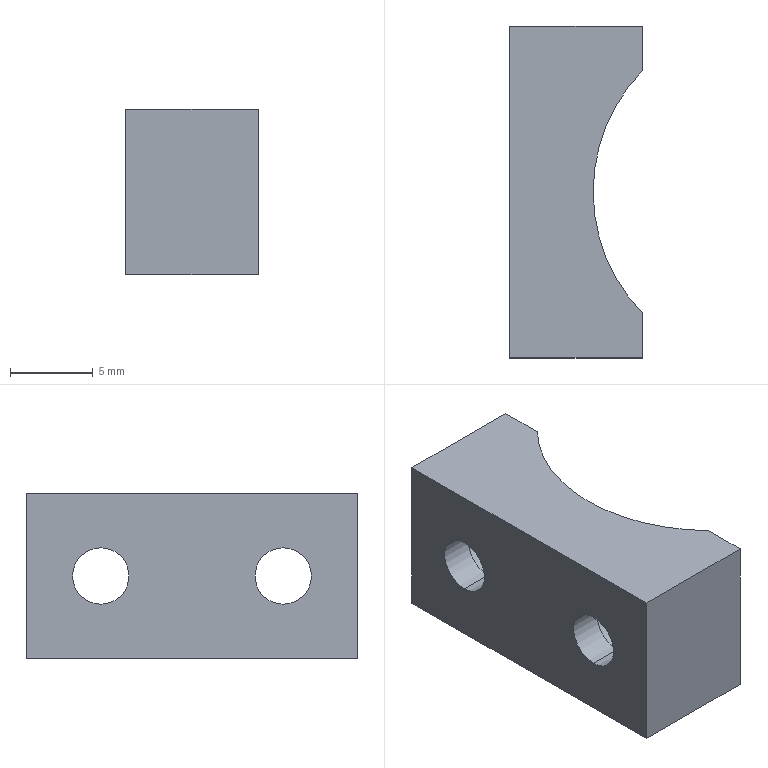Part | SolidWorks | features Extrusion 1, HoleWzd 1, RevCut 1 | 1 solid | 19 faces | box 8 x 20 x 10 mm | volume 974.548 mm3 | plane 9 | cylinder 8 | cone 2 | commonest cylinder face diameters 3.4 x4 6 x4
STEP:
#1=CARTESIAN_POINT('',(1.034,0.,10.));
#2=VERTEX_POINT('',#1);
#3=CARTESIAN_POINT('',(4.,7.299,10.));
#4=VERTEX_POINT('',#3);
#5=CARTESIAN_POINT('',(11.5,0.,10.));
#6=DIRECTION('',(0.,0.,-1.));
#7=DIRECTION('',(1.,0.,0.));
#8=AXIS2_PLACEMENT_3D('',#5,#6,#7);
#9=CIRCLE('',#8,10.466);
#10=EDGE_CURVE('',#2,#4,#9,.T.);
#11=ORIENTED_EDGE('',*,*,#10,.F.);
#12=CARTESIAN_POINT('',(0.5697,0.,0.));
#13=VERTEX_POINT('',#12);
#14=CARTESIAN_POINT('',(0.5,0.,-1.5));
#15=DIRECTION('',(-0.04641,0.,-0.9989));
#16=VECTOR('',#15,1000.);
#17=LINE('',#14,#16);
#18=EDGE_CURVE('',#2,#13,#17,.T.);
#19=ORIENTED_EDGE('',*,*,#18,.T.);
#20=CARTESIAN_POINT('',(4.,7.951,0.));
#21=VERTEX_POINT('',#20);
#22=CARTESIAN_POINT('',(11.5,0.,0.));
#23=DIRECTION('',(0.,0.,-1.));
#24=DIRECTION('',(1.,0.,0.));
#25=AXIS2_PLACEMENT_3D('',#22,#23,#24);
#26=CIRCLE('',#25,10.93);
#27=EDGE_CURVE('',#13,#21,#26,.T.);
#28=ORIENTED_EDGE('',*,*,#27,.T.);
#29=CARTESIAN_POINT('',(4.,7.757,3.024));
#30=VERTEX_POINT('',#29);
#31=CARTESIAN_POINT('',(4.,7.951,0.));
#32=CARTESIAN_POINT('',(4.,7.887,1.008));
#33=CARTESIAN_POINT('',(4.,7.822,2.016));
#34=CARTESIAN_POINT('',(4.,7.757,3.024));
#35=B_SPLINE_CURVE_WITH_KNOTS('',3,(#31,#32,#33,#34),.UNSPECIFIED.,.F.,.F.,(4,4),(0.0224,0.02543),.UNSPECIFIED.);
#36=EDGE_CURVE('',#21,#30,#35,.T.);
#37=ORIENTED_EDGE('',*,*,#36,.T.);
#38=CARTESIAN_POINT('',(2.162,5.5,2.));
#39=VERTEX_POINT('',#38);
#40=CARTESIAN_POINT('',(4.,7.757,3.024));
#41=CARTESIAN_POINT('',(3.843,7.616,2.863));
#42=CARTESIAN_POINT('',(3.684,7.463,2.722));
#43=CARTESIAN_POINT('',(3.365,7.131,2.473));
#44=CARTESIAN_POINT('',(3.204,6.952,2.366));
#45=CARTESIAN_POINT('',(2.887,6.568,2.188));
#46=CARTESIAN_POINT('',(2.733,6.367,2.12));
#47=CARTESIAN_POINT('',(2.439,5.948,2.026));
#48=CARTESIAN_POINT('',(2.297,5.729,2.));
#49=CARTESIAN_POINT('',(2.162,5.5,2.));
#50=B_SPLINE_CURVE_WITH_KNOTS('',3,(#40,#41,#42,#43,#44,#45,#46,#47,#48,#49),.UNSPECIFIED.,.F.,.F.,(4,2,2,2,4),(0.000000334,0.0007849,0.00157,0.002354,0.003139),.UNSPECIFIED.);
#51=EDGE_CURVE('',#30,#39,#50,.T.);
#52=ORIENTED_EDGE('',*,*,#51,.T.);
#53=CARTESIAN_POINT('',(2.487,5.5,8.));
#54=VERTEX_POINT('',#53);
#55=CARTESIAN_POINT('',(2.162,5.5,2.));
#56=CARTESIAN_POINT('',(2.057,5.322,2.));
#57=CARTESIAN_POINT('',(1.959,5.142,2.016));
#58=CARTESIAN_POINT('',(1.777,4.782,2.082));
#59=CARTESIAN_POINT('',(1.691,4.599,2.132));
#60=CARTESIAN_POINT('',(1.539,4.241,2.27));
#61=CARTESIAN_POINT('',(1.472,4.069,2.356));
#62=CARTESIAN_POINT('',(1.354,3.737,2.565));
#63=CARTESIAN_POINT('',(1.303,3.577,2.689));
#64=CARTESIAN_POINT('',(1.219,3.285,2.967));
#65=CARTESIAN_POINT('',(1.185,3.154,3.12));
#66=CARTESIAN_POINT('',(1.133,2.92,3.455));
#67=CARTESIAN_POINT('',(1.114,2.82,3.637));
#68=CARTESIAN_POINT('',(1.09,2.659,4.014));
#69=CARTESIAN_POINT('',(1.084,2.598,4.212));
#70=CARTESIAN_POINT('',(1.084,2.517,4.618));
#71=CARTESIAN_POINT('',(1.089,2.498,4.822));
#72=CARTESIAN_POINT('',(1.11,2.502,5.232));
#73=CARTESIAN_POINT('',(1.125,2.525,5.44));
#74=CARTESIAN_POINT('',(1.166,2.612,5.839));
#75=CARTESIAN_POINT('',(1.191,2.676,6.033));
#76=CARTESIAN_POINT('',(1.254,2.843,6.408));
#77=CARTESIAN_POINT('',(1.291,2.944,6.583));
#78=CARTESIAN_POINT('',(1.377,3.177,6.909));
#79=CARTESIAN_POINT('',(1.427,3.311,7.061));
#80=CARTESIAN_POINT('',(1.54,3.601,7.331));
#81=CARTESIAN_POINT('',(1.603,3.757,7.449));
#82=CARTESIAN_POINT('',(1.745,4.086,7.653));
#83=CARTESIAN_POINT('',(1.823,4.259,7.738));
#84=CARTESIAN_POINT('',(2.076,4.784,7.937));
#85=CARTESIAN_POINT('',(2.273,5.15,8.));
#86=CARTESIAN_POINT('',(2.487,5.5,8.));
#87=B_SPLINE_CURVE_WITH_KNOTS('',3,(#55,#56,#57,#58,#59,#60,#61,#62,#63,#64,#65,#66,#67,#68,#69,#70,#71,#72,#73,#74,#75,#76,#77,#78,#79,#80,#81,#82,#83,#84,#85,#86),.UNSPECIFIED.,.F.,.F.,(4,2,2,2,2,2,2,2,2,2,2,2,2,2,2,4),(0.003139,0.003751,0.004363,0.004975,0.005588,0.0062,0.006812,0.007424,0.008037,0.008649,0.009261,0.009873,0.01049,0.0111,0.01171,0.01293),.UNSPECIFIED.);
#88=EDGE_CURVE('',#39,#54,#87,.T.);
#89=ORIENTED_EDGE('',*,*,#88,.T.);
#90=CARTESIAN_POINT('',(4.,7.481,7.253));
#91=VERTEX_POINT('',#90);
#92=CARTESIAN_POINT('',(2.487,5.5,8.));
#93=CARTESIAN_POINT('',(2.601,5.687,8.));
#94=CARTESIAN_POINT('',(2.722,5.873,7.982));
#95=CARTESIAN_POINT('',(2.969,6.231,7.915));
#96=CARTESIAN_POINT('',(3.095,6.404,7.866));
#97=CARTESIAN_POINT('',(3.351,6.736,7.739));
#98=CARTESIAN_POINT('',(3.482,6.897,7.661));
#99=CARTESIAN_POINT('',(3.743,7.202,7.477));
#100=CARTESIAN_POINT('',(3.872,7.345,7.372));
#101=CARTESIAN_POINT('',(4.,7.481,7.253));
#102=B_SPLINE_CURVE_WITH_KNOTS('',3,(#92,#93,#94,#95,#96,#97,#98,#99,#100,#101),.UNSPECIFIED.,.F.,.F.,(4,2,2,2,4),(0.01293,0.01359,0.01424,0.0149,0.01555),.UNSPECIFIED.);
#103=EDGE_CURVE('',#54,#91,#102,.T.);
#104=ORIENTED_EDGE('',*,*,#103,.T.);
#105=CARTESIAN_POINT('',(4.,7.481,7.253));
#106=CARTESIAN_POINT('',(4.,7.421,8.168));
#107=CARTESIAN_POINT('',(4.,7.36,9.084));
#108=CARTESIAN_POINT('',(4.,7.299,10.));
#109=B_SPLINE_CURVE_WITH_KNOTS('',3,(#105,#106,#107,#108),.UNSPECIFIED.,.F.,.F.,(4,4),(0.02967,0.03242),.UNSPECIFIED.);
#110=EDGE_CURVE('',#91,#4,#109,.T.);
#111=ORIENTED_EDGE('',*,*,#110,.T.);
#112=EDGE_LOOP('',(#11,#19,#28,#37,#52,#89,#104,#111));
#113=FACE_OUTER_BOUND('',#112,.T.);
#114=CARTESIAN_POINT('',(11.5,0.,-1.5));
#115=DIRECTION('',(0.,0.,-1.));
#116=DIRECTION('',(-1.,0.,0.));
#117=AXIS2_PLACEMENT_3D('',#114,#115,#116);
#118=CONICAL_SURFACE('',#117,11.,0.04643);
#119=ADVANCED_FACE('',(#113),#118,.F.);
#120=CARTESIAN_POINT('',(-4.,5.5,6.7));
#121=VERTEX_POINT('',#120);
#122=CARTESIAN_POINT('',(-4.,5.5,3.3));
#123=VERTEX_POINT('',#122);
#124=CARTESIAN_POINT('',(-4.,5.5,5.));
#125=DIRECTION('',(1.,0.,0.));
#126=DIRECTION('',(0.,0.,-1.));
#127=AXIS2_PLACEMENT_3D('',#124,#125,#126);
#128=CIRCLE('',#127,1.7);
#129=EDGE_CURVE('',#121,#123,#128,.T.);
#130=ORIENTED_EDGE('',*,*,#129,.F.);
#131=CARTESIAN_POINT('',(-2.,5.5,6.7));
#132=VERTEX_POINT('',#131);
#133=CARTESIAN_POINT('',(4.,5.5,6.7));
#134=DIRECTION('',(1.,0.,0.));
#135=VECTOR('',#134,1000.);
#136=LINE('',#133,#135);
#137=EDGE_CURVE('',#121,#132,#136,.T.);
#138=ORIENTED_EDGE('',*,*,#137,.T.);
#139=CARTESIAN_POINT('',(-2.,5.5,3.3));
#140=VERTEX_POINT('',#139);
#141=CARTESIAN_POINT('',(-2.,5.5,5.));
#142=DIRECTION('',(1.,0.,0.));
#143=DIRECTION('',(0.,0.,-1.));
#144=AXIS2_PLACEMENT_3D('',#141,#142,#143);
#145=CIRCLE('',#144,1.7);
#146=EDGE_CURVE('',#132,#140,#145,.T.);
#147=ORIENTED_EDGE('',*,*,#146,.T.);
#148=CARTESIAN_POINT('',(4.,5.5,3.3));
#149=DIRECTION('',(1.,0.,0.));
#150=VECTOR('',#149,1000.);
#151=LINE('',#148,#150);
#152=EDGE_CURVE('',#123,#140,#151,.T.);
#153=ORIENTED_EDGE('',*,*,#152,.F.);
#154=EDGE_LOOP('',(#130,#138,#147,#153));
#155=FACE_OUTER_BOUND('',#154,.T.);
#156=CARTESIAN_POINT('',(4.,5.5,5.));
#157=DIRECTION('',(1.,0.,0.));
#158=DIRECTION('',(0.,0.,-1.));
#159=AXIS2_PLACEMENT_3D('',#156,#157,#158);
#160=CYLINDRICAL_SURFACE('',#159,1.7);
#161=ADVANCED_FACE('',(#155),#160,.F.);
#162=CARTESIAN_POINT('',(-4.,-5.5,6.7));
#163=VERTEX_POINT('',#162);
#164=CARTESIAN_POINT('',(-4.,-5.5,3.3));
#165=VERTEX_POINT('',#164);
#166=CARTESIAN_POINT('',(-4.,-5.5,5.));
#167=DIRECTION('',(1.,0.,0.));
#168=DIRECTION('',(0.,0.,-1.));
#169=AXIS2_PLACEMENT_3D('',#166,#167,#168);
#170=CIRCLE('',#169,1.7);
#171=EDGE_CURVE('',#163,#165,#170,.T.);
#172=ORIENTED_EDGE('',*,*,#171,.F.);
#173=CARTESIAN_POINT('',(-2.,-5.5,6.7));
#174=VERTEX_POINT('',#173);
#175=CARTESIAN_POINT('',(4.,-5.5,6.7));
#176=DIRECTION('',(1.,0.,0.));
#177=VECTOR('',#176,1000.);
#178=LINE('',#175,#177);
#179=EDGE_CURVE('',#163,#174,#178,.T.);
#180=ORIENTED_EDGE('',*,*,#179,.T.);
#181=CARTESIAN_POINT('',(-2.,-5.5,3.3));
#182=VERTEX_POINT('',#181);
#183=CARTESIAN_POINT('',(-2.,-5.5,5.));
#184=DIRECTION('',(1.,0.,0.));
#185=DIRECTION('',(0.,0.,-1.));
#186=AXIS2_PLACEMENT_3D('',#183,#184,#185);
#187=CIRCLE('',#186,1.7);
#188=EDGE_CURVE('',#174,#182,#187,.T.);
#189=ORIENTED_EDGE('',*,*,#188,.T.);
#190=CARTESIAN_POINT('',(4.,-5.5,3.3));
#191=DIRECTION('',(1.,0.,0.));
#192=VECTOR('',#191,1000.);
#193=LINE('',#190,#192);
#194=EDGE_CURVE('',#165,#182,#193,.T.);
#195=ORIENTED_EDGE('',*,*,#194,.F.);
#196=EDGE_LOOP('',(#172,#180,#189,#195));
#197=FACE_OUTER_BOUND('',#196,.T.);
#198=CARTESIAN_POINT('',(4.,-5.5,5.));
#199=DIRECTION('',(1.,0.,0.));
#200=DIRECTION('',(0.,0.,-1.));
#201=AXIS2_PLACEMENT_3D('',#198,#199,#200);
#202=CYLINDRICAL_SURFACE('',#201,1.7);
#203=ADVANCED_FACE('',(#197),#202,.F.);
#204=CARTESIAN_POINT('',(-2.,5.5,8.));
#205=VERTEX_POINT('',#204);
#206=CARTESIAN_POINT('',(-2.,5.5,2.));
#207=VERTEX_POINT('',#206);
#208=CARTESIAN_POINT('',(-2.,5.5,5.));
#209=DIRECTION('',(1.,0.,0.));
#210=DIRECTION('',(0.,0.,-1.));
#211=AXIS2_PLACEMENT_3D('',#208,#209,#210);
#212=CIRCLE('',#211,3.);
#213=EDGE_CURVE('',#205,#207,#212,.T.);
#214=ORIENTED_EDGE('',*,*,#213,.F.);
#215=CARTESIAN_POINT('',(4.,5.5,8.));
#216=DIRECTION('',(1.,0.,0.));
#217=VECTOR('',#216,1000.);
#218=LINE('',#215,#217);
#219=EDGE_CURVE('',#205,#54,#218,.T.);
#220=ORIENTED_EDGE('',*,*,#219,.T.);
#221=ORIENTED_EDGE('',*,*,#88,.F.);
#222=CARTESIAN_POINT('',(4.,5.5,2.));
#223=DIRECTION('',(1.,0.,0.));
#224=VECTOR('',#223,1000.);
#225=LINE('',#222,#224);
#226=EDGE_CURVE('',#207,#39,#225,.T.);
#227=ORIENTED_EDGE('',*,*,#226,.F.);
#228=EDGE_LOOP('',(#214,#220,#221,#227));
#229=FACE_OUTER_BOUND('',#228,.T.);
#230=CARTESIAN_POINT('',(4.,5.5,5.));
#231=DIRECTION('',(1.,0.,0.));
#232=DIRECTION('',(0.,0.,-1.));
#233=AXIS2_PLACEMENT_3D('',#230,#231,#232);
#234=CYLINDRICAL_SURFACE('',#233,3.);
#235=ADVANCED_FACE('',(#229),#234,.F.);
#236=CARTESIAN_POINT('',(-2.,-5.5,8.));
#237=VERTEX_POINT('',#236);
#238=CARTESIAN_POINT('',(-2.,-5.5,2.));
#239=VERTEX_POINT('',#238);
#240=CARTESIAN_POINT('',(-2.,-5.5,5.));
#241=DIRECTION('',(1.,0.,0.));
#242=DIRECTION('',(0.,0.,-1.));
#243=AXIS2_PLACEMENT_3D('',#240,#241,#242);
#244=CIRCLE('',#243,3.);
#245=EDGE_CURVE('',#237,#239,#244,.T.);
#246=ORIENTED_EDGE('',*,*,#245,.F.);
#247=CARTESIAN_POINT('',(2.487,-5.5,8.));
#248=VERTEX_POINT('',#247);
#249=CARTESIAN_POINT('',(4.,-5.5,8.));
#250=DIRECTION('',(1.,0.,0.));
#251=VECTOR('',#250,1000.);
#252=LINE('',#249,#251);
#253=EDGE_CURVE('',#237,#248,#252,.T.);
#254=ORIENTED_EDGE('',*,*,#253,.T.);
#255=CARTESIAN_POINT('',(4.,-7.481,7.253));
#256=VERTEX_POINT('',#255);
#257=CARTESIAN_POINT('',(4.,-7.481,7.253));
#258=CARTESIAN_POINT('',(3.743,-7.208,7.493));
#259=CARTESIAN_POINT('',(3.482,-6.906,7.674));
#260=CARTESIAN_POINT('',(3.094,-6.404,7.866));
#261=CARTESIAN_POINT('',(2.966,-6.228,7.916));
#262=CARTESIAN_POINT('',(2.72,-5.87,7.983));
#263=CARTESIAN_POINT('',(2.601,-5.687,8.));
#264=CARTESIAN_POINT('',(2.487,-5.5,8.));
#265=B_SPLINE_CURVE_WITH_KNOTS('',3,(#257,#258,#259,#260,#261,#262,#263,#264),.UNSPECIFIED.,.F.,.F.,(4,2,2,4),(0.000000342,0.001317,0.001975,0.002633),.UNSPECIFIED.);
#266=EDGE_CURVE('',#256,#248,#265,.T.);
#267=ORIENTED_EDGE('',*,*,#266,.F.);
#268=CARTESIAN_POINT('',(4.,-7.757,3.024));
#269=VERTEX_POINT('',#268);
#270=CARTESIAN_POINT('',(4.,-5.5,5.));
#271=DIRECTION('',(1.,0.,0.));
#272=DIRECTION('',(0.,0.,-1.));
#273=AXIS2_PLACEMENT_3D('',#270,#271,#272);
#274=CIRCLE('',#273,3.);
#275=EDGE_CURVE('',#256,#269,#274,.T.);
#276=ORIENTED_EDGE('',*,*,#275,.T.);
#277=CARTESIAN_POINT('',(2.162,-5.5,2.));
#278=VERTEX_POINT('',#277);
#279=CARTESIAN_POINT('',(2.162,-5.5,2.));
#280=CARTESIAN_POINT('',(2.295,-5.726,2.));
#281=CARTESIAN_POINT('',(2.437,-5.945,2.025));
#282=CARTESIAN_POINT('',(2.734,-6.368,2.12));
#283=CARTESIAN_POINT('',(2.889,-6.571,2.19));
#284=CARTESIAN_POINT('',(3.36,-7.139,2.453));
#285=CARTESIAN_POINT('',(3.688,-7.476,2.703));
#286=CARTESIAN_POINT('',(4.,-7.757,3.024));
#287=B_SPLINE_CURVE_WITH_KNOTS('',3,(#279,#280,#281,#282,#283,#284,#285,#286),.UNSPECIFIED.,.F.,.F.,(4,2,2,4),(0.01242,0.0132,0.01398,0.01554),.UNSPECIFIED.);
#288=EDGE_CURVE('',#278,#269,#287,.T.);
#289=ORIENTED_EDGE('',*,*,#288,.F.);
#290=CARTESIAN_POINT('',(4.,-5.5,2.));
#291=DIRECTION('',(1.,0.,0.));
#292=VECTOR('',#291,1000.);
#293=LINE('',#290,#292);
#294=EDGE_CURVE('',#239,#278,#293,.T.);
#295=ORIENTED_EDGE('',*,*,#294,.F.);
#296=EDGE_LOOP('',(#246,#254,#267,#276,#289,#295));
#297=FACE_OUTER_BOUND('',#296,.T.);
#298=CARTESIAN_POINT('',(4.,-5.5,5.));
#299=DIRECTION('',(1.,0.,0.));
#300=DIRECTION('',(0.,0.,-1.));
#301=AXIS2_PLACEMENT_3D('',#298,#299,#300);
#302=CYLINDRICAL_SURFACE('',#301,3.);
#303=ADVANCED_FACE('',(#297),#302,.F.);
#304=CARTESIAN_POINT('',(4.,-7.299,10.));
#305=VERTEX_POINT('',#304);
#306=CARTESIAN_POINT('',(4.,-7.299,10.));
#307=CARTESIAN_POINT('',(4.,-7.36,9.084));
#308=CARTESIAN_POINT('',(4.,-7.421,8.168));
#309=CARTESIAN_POINT('',(4.,-7.481,7.253));
#310=B_SPLINE_CURVE_WITH_KNOTS('',3,(#306,#307,#308,#309),.UNSPECIFIED.,.F.,.F.,(4,4),(0.02242,0.02517),.UNSPECIFIED.);
#311=EDGE_CURVE('',#305,#256,#310,.T.);
#312=ORIENTED_EDGE('',*,*,#311,.F.);
#313=CARTESIAN_POINT('',(4.,-10.,10.));
#314=VERTEX_POINT('',#313);
#315=CARTESIAN_POINT('',(4.,10.,10.));
#316=DIRECTION('',(0.,1.,0.));
#317=VECTOR('',#316,1000.);
#318=LINE('',#315,#317);
#319=EDGE_CURVE('',#314,#305,#318,.T.);
#320=ORIENTED_EDGE('',*,*,#319,.F.);
#321=CARTESIAN_POINT('',(4.,-10.,0.));
#322=VERTEX_POINT('',#321);
#323=CARTESIAN_POINT('',(4.,-10.,10.));
#324=DIRECTION('',(0.,0.,-1.));
#325=VECTOR('',#324,1000.);
#326=LINE('',#323,#325);
#327=EDGE_CURVE('',#314,#322,#326,.T.);
#328=ORIENTED_EDGE('',*,*,#327,.T.);
#329=CARTESIAN_POINT('',(4.,-7.951,0.));
#330=VERTEX_POINT('',#329);
#331=CARTESIAN_POINT('',(4.,10.,0.));
#332=DIRECTION('',(0.,1.,0.));
#333=VECTOR('',#332,1000.);
#334=LINE('',#331,#333);
#335=EDGE_CURVE('',#322,#330,#334,.T.);
#336=ORIENTED_EDGE('',*,*,#335,.T.);
#337=CARTESIAN_POINT('',(4.,-7.757,3.024));
#338=CARTESIAN_POINT('',(4.,-7.822,2.016));
#339=CARTESIAN_POINT('',(4.,-7.887,1.008));
#340=CARTESIAN_POINT('',(4.,-7.951,0.));
#341=B_SPLINE_CURVE_WITH_KNOTS('',3,(#337,#338,#339,#340),.UNSPECIFIED.,.F.,.F.,(4,4),(0.02941,0.03244),.UNSPECIFIED.);
#342=EDGE_CURVE('',#269,#330,#341,.T.);
#343=ORIENTED_EDGE('',*,*,#342,.F.);
#344=ORIENTED_EDGE('',*,*,#275,.F.);
#345=EDGE_LOOP('',(#312,#320,#328,#336,#343,#344));
#346=FACE_OUTER_BOUND('',#345,.T.);
#347=CARTESIAN_POINT('',(4.,10.,10.));
#348=DIRECTION('',(-1.,0.,0.));
#349=DIRECTION('',(0.,-1.,0.));
#350=AXIS2_PLACEMENT_3D('',#347,#348,#349);
#351=PLANE('',#350);
#352=ADVANCED_FACE('',(#346),#351,.F.);
#353=ORIENTED_EDGE('',*,*,#36,.F.);
#354=CARTESIAN_POINT('',(4.,10.,0.));
#355=VERTEX_POINT('',#354);
#356=CARTESIAN_POINT('',(4.,10.,0.));
#357=DIRECTION('',(0.,1.,0.));
#358=VECTOR('',#357,1000.);
#359=LINE('',#356,#358);
#360=EDGE_CURVE('',#21,#355,#359,.T.);
#361=ORIENTED_EDGE('',*,*,#360,.T.);
#362=CARTESIAN_POINT('',(4.,10.,10.));
#363=VERTEX_POINT('',#362);
#364=CARTESIAN_POINT('',(4.,10.,10.));
#365=DIRECTION('',(0.,0.,-1.));
#366=VECTOR('',#365,1000.);
#367=LINE('',#364,#366);
#368=EDGE_CURVE('',#363,#355,#367,.T.);
#369=ORIENTED_EDGE('',*,*,#368,.F.);
#370=CARTESIAN_POINT('',(4.,10.,10.));
#371=DIRECTION('',(0.,1.,0.));
#372=VECTOR('',#371,1000.);
#373=LINE('',#370,#372);
#374=EDGE_CURVE('',#4,#363,#373,.T.);
#375=ORIENTED_EDGE('',*,*,#374,.F.);
#376=ORIENTED_EDGE('',*,*,#110,.F.);
#377=CARTESIAN_POINT('',(4.,5.5,5.));
#378=DIRECTION('',(1.,0.,0.));
#379=DIRECTION('',(0.,0.,-1.));
#380=AXIS2_PLACEMENT_3D('',#377,#378,#379);
#381=CIRCLE('',#380,3.);
#382=EDGE_CURVE('',#30,#91,#381,.T.);
#383=ORIENTED_EDGE('',*,*,#382,.F.);
#384=EDGE_LOOP('',(#353,#361,#369,#375,#376,#383));
#385=FACE_OUTER_BOUND('',#384,.T.);
#386=CARTESIAN_POINT('',(4.,10.,10.));
#387=DIRECTION('',(-1.,0.,0.));
#388=DIRECTION('',(0.,-1.,0.));
#389=AXIS2_PLACEMENT_3D('',#386,#387,#388);
#390=PLANE('',#389);
#391=ADVANCED_FACE('',(#385),#390,.F.);
#392=ORIENTED_EDGE('',*,*,#253,.F.);
#393=CARTESIAN_POINT('',(-2.,-5.5,5.));
#394=DIRECTION('',(1.,0.,0.));
#395=DIRECTION('',(0.,0.,-1.));
#396=AXIS2_PLACEMENT_3D('',#393,#394,#395);
#397=CIRCLE('',#396,3.);
#398=EDGE_CURVE('',#239,#237,#397,.T.);
#399=ORIENTED_EDGE('',*,*,#398,.F.);
#400=ORIENTED_EDGE('',*,*,#294,.T.);
#401=CARTESIAN_POINT('',(2.487,-5.5,8.));
#402=CARTESIAN_POINT('',(2.381,-5.326,8.));
#403=CARTESIAN_POINT('',(2.277,-5.146,7.985));
#404=CARTESIAN_POINT('',(2.083,-4.788,7.92));
#405=CARTESIAN_POINT('',(1.993,-4.611,7.871));
#406=CARTESIAN_POINT('',(1.824,-4.262,7.739));
#407=CARTESIAN_POINT('',(1.746,-4.087,7.654));
#408=CARTESIAN_POINT('',(1.605,-3.76,7.451));
#409=CARTESIAN_POINT('',(1.542,-3.605,7.334));
#410=CARTESIAN_POINT('',(1.429,-3.316,7.066));
#411=CARTESIAN_POINT('',(1.378,-3.181,6.913));
#412=CARTESIAN_POINT('',(1.292,-2.947,6.588));
#413=CARTESIAN_POINT('',(1.255,-2.846,6.414));
#414=CARTESIAN_POINT('',(1.192,-2.679,6.04));
#415=CARTESIAN_POINT('',(1.167,-2.614,5.845));
#416=CARTESIAN_POINT('',(1.126,-2.527,5.447));
#417=CARTESIAN_POINT('',(1.11,-2.503,5.241));
#418=CARTESIAN_POINT('',(1.089,-2.498,4.829));
#419=CARTESIAN_POINT('',(1.084,-2.516,4.625));
#420=CARTESIAN_POINT('',(1.084,-2.596,4.221));
#421=CARTESIAN_POINT('',(1.09,-2.657,4.021));
#422=CARTESIAN_POINT('',(1.114,-2.816,3.644));
#423=CARTESIAN_POINT('',(1.132,-2.915,3.464));
#424=CARTESIAN_POINT('',(1.184,-3.149,3.125));
#425=CARTESIAN_POINT('',(1.217,-3.281,2.971));
#426=CARTESIAN_POINT('',(1.301,-3.571,2.694));
#427=CARTESIAN_POINT('',(1.352,-3.731,2.569));
#428=CARTESIAN_POINT('',(1.47,-4.064,2.359));
#429=CARTESIAN_POINT('',(1.537,-4.238,2.272));
#430=CARTESIAN_POINT('',(1.691,-4.597,2.133));
#431=CARTESIAN_POINT('',(1.775,-4.778,2.082));
#432=CARTESIAN_POINT('',(1.958,-5.14,2.016));
#433=CARTESIAN_POINT('',(2.057,-5.322,2.));
#434=CARTESIAN_POINT('',(2.162,-5.5,2.));
#435=B_SPLINE_CURVE_WITH_KNOTS('',3,(#401,#402,#403,#404,#405,#406,#407,#408,#409,#410,#411,#412,#413,#414,#415,#416,#417,#418,#419,#420,#421,#422,#423,#424,#425,#426,#427,#428,#429,#430,#431,#432,#433,#434),.UNSPECIFIED.,.F.,.F.,(4,2,2,2,2,2,2,2,2,2,2,2,2,2,2,2,4),(0.002633,0.003245,0.003857,0.004469,0.00508,0.005692,0.006304,0.006916,0.007528,0.00814,0.008752,0.009364,0.009976,0.01059,0.0112,0.01181,0.01242),.UNSPECIFIED.);
#436=EDGE_CURVE('',#248,#278,#435,.T.);
#437=ORIENTED_EDGE('',*,*,#436,.F.);
#438=EDGE_LOOP('',(#392,#399,#400,#437));
#439=FACE_OUTER_BOUND('',#438,.T.);
#440=CARTESIAN_POINT('',(4.,-5.5,5.));
#441=DIRECTION('',(1.,0.,0.));
#442=DIRECTION('',(0.,0.,-1.));
#443=AXIS2_PLACEMENT_3D('',#440,#441,#442);
#444=CYLINDRICAL_SURFACE('',#443,3.);
#445=ADVANCED_FACE('',(#439),#444,.F.);
#446=ORIENTED_EDGE('',*,*,#219,.F.);
#447=CARTESIAN_POINT('',(-2.,5.5,5.));
#448=DIRECTION('',(1.,0.,0.));
#449=DIRECTION('',(0.,0.,-1.));
#450=AXIS2_PLACEMENT_3D('',#447,#448,#449);
#451=CIRCLE('',#450,3.);
#452=EDGE_CURVE('',#207,#205,#451,.T.);
#453=ORIENTED_EDGE('',*,*,#452,.F.);
#454=ORIENTED_EDGE('',*,*,#226,.T.);
#455=ORIENTED_EDGE('',*,*,#51,.F.);
#456=ORIENTED_EDGE('',*,*,#382,.T.);
#457=ORIENTED_EDGE('',*,*,#103,.F.);
#458=EDGE_LOOP('',(#446,#453,#454,#455,#456,#457));
#459=FACE_OUTER_BOUND('',#458,.T.);
#460=CARTESIAN_POINT('',(4.,5.5,5.));
#461=DIRECTION('',(1.,0.,0.));
#462=DIRECTION('',(0.,0.,-1.));
#463=AXIS2_PLACEMENT_3D('',#460,#461,#462);
#464=CYLINDRICAL_SURFACE('',#463,3.);
#465=ADVANCED_FACE('',(#459),#464,.F.);
#466=CARTESIAN_POINT('',(-4.,10.,0.));
#467=VERTEX_POINT('',#466);
#468=CARTESIAN_POINT('',(-4.,10.,0.));
#469=DIRECTION('',(-1.,0.,0.));
#470=VECTOR('',#469,1000.);
#471=LINE('',#468,#470);
#472=EDGE_CURVE('',#355,#467,#471,.T.);
#473=ORIENTED_EDGE('',*,*,#472,.T.);
#474=CARTESIAN_POINT('',(-4.,10.,10.));
#475=VERTEX_POINT('',#474);
#476=CARTESIAN_POINT('',(-4.,10.,10.));
#477=DIRECTION('',(0.,0.,-1.));
#478=VECTOR('',#477,1000.);
#479=LINE('',#476,#478);
#480=EDGE_CURVE('',#475,#467,#479,.T.);
#481=ORIENTED_EDGE('',*,*,#480,.F.);
#482=CARTESIAN_POINT('',(-4.,10.,10.));
#483=DIRECTION('',(-1.,0.,0.));
#484=VECTOR('',#483,1000.);
#485=LINE('',#482,#484);
#486=EDGE_CURVE('',#363,#475,#485,.T.);
#487=ORIENTED_EDGE('',*,*,#486,.F.);
#488=ORIENTED_EDGE('',*,*,#368,.T.);
#489=EDGE_LOOP('',(#473,#481,#487,#488));
#490=FACE_OUTER_BOUND('',#489,.T.);
#491=CARTESIAN_POINT('',(-4.,10.,10.));
#492=DIRECTION('',(0.,-1.,0.));
#493=DIRECTION('',(0.,0.,-1.));
#494=AXIS2_PLACEMENT_3D('',#491,#492,#493);
#495=PLANE('',#494);
#496=ADVANCED_FACE('',(#490),#495,.F.);
#497=CARTESIAN_POINT('',(-4.,5.5,5.));
#498=DIRECTION('',(1.,0.,0.));
#499=DIRECTION('',(0.,0.,-1.));
#500=AXIS2_PLACEMENT_3D('',#497,#498,#499);
#501=CIRCLE('',#500,1.7);
#502=EDGE_CURVE('',#123,#121,#501,.T.);
#503=ORIENTED_EDGE('',*,*,#502,.T.);
#504=ORIENTED_EDGE('',*,*,#129,.T.);
#505=EDGE_LOOP('',(#503,#504));
#506=FACE_BOUND('',#505,.T.);
#507=CARTESIAN_POINT('',(-4.,-5.5,5.));
#508=DIRECTION('',(1.,0.,0.));
#509=DIRECTION('',(0.,0.,-1.));
#510=AXIS2_PLACEMENT_3D('',#507,#508,#509);
#511=CIRCLE('',#510,1.7);
#512=EDGE_CURVE('',#165,#163,#511,.T.);
#513=ORIENTED_EDGE('',*,*,#512,.T.);
#514=ORIENTED_EDGE('',*,*,#171,.T.);
#515=EDGE_LOOP('',(#513,#514));
#516=FACE_BOUND('',#515,.T.);
#517=CARTESIAN_POINT('',(-4.,-10.,0.));
#518=VERTEX_POINT('',#517);
#519=CARTESIAN_POINT('',(-4.,10.,0.));
#520=DIRECTION('',(0.,-1.,0.));
#521=VECTOR('',#520,1000.);
#522=LINE('',#519,#521);
#523=EDGE_CURVE('',#467,#518,#522,.T.);
#524=ORIENTED_EDGE('',*,*,#523,.T.);
#525=CARTESIAN_POINT('',(-4.,-10.,10.));
#526=VERTEX_POINT('',#525);
#527=CARTESIAN_POINT('',(-4.,-10.,10.));
#528=DIRECTION('',(0.,0.,-1.));
#529=VECTOR('',#528,1000.);
#530=LINE('',#527,#529);
#531=EDGE_CURVE('',#526,#518,#530,.T.);
#532=ORIENTED_EDGE('',*,*,#531,.F.);
#533=CARTESIAN_POINT('',(-4.,10.,10.));
#534=DIRECTION('',(0.,-1.,0.));
#535=VECTOR('',#534,1000.);
#536=LINE('',#533,#535);
#537=EDGE_CURVE('',#475,#526,#536,.T.);
#538=ORIENTED_EDGE('',*,*,#537,.F.);
#539=ORIENTED_EDGE('',*,*,#480,.T.);
#540=EDGE_LOOP('',(#524,#532,#538,#539));
#541=FACE_OUTER_BOUND('',#540,.T.);
#542=CARTESIAN_POINT('',(-4.,10.,10.));
#543=DIRECTION('',(1.,0.,0.));
#544=DIRECTION('',(0.,1.,0.));
#545=AXIS2_PLACEMENT_3D('',#542,#543,#544);
#546=PLANE('',#545);
#547=ADVANCED_FACE('',(#506,#516,#541),#546,.F.);
#548=CARTESIAN_POINT('',(-4.,-10.,0.));
#549=DIRECTION('',(1.,0.,0.));
#550=VECTOR('',#549,1000.);
#551=LINE('',#548,#550);
#552=EDGE_CURVE('',#518,#322,#551,.T.);
#553=ORIENTED_EDGE('',*,*,#552,.T.);
#554=ORIENTED_EDGE('',*,*,#327,.F.);
#555=CARTESIAN_POINT('',(-4.,-10.,10.));
#556=DIRECTION('',(1.,0.,0.));
#557=VECTOR('',#556,1000.);
#558=LINE('',#555,#557);
#559=EDGE_CURVE('',#526,#314,#558,.T.);
#560=ORIENTED_EDGE('',*,*,#559,.F.);
#561=ORIENTED_EDGE('',*,*,#531,.T.);
#562=EDGE_LOOP('',(#553,#554,#560,#561));
#563=FACE_OUTER_BOUND('',#562,.T.);
#564=CARTESIAN_POINT('',(-4.,-10.,10.));
#565=DIRECTION('',(0.,1.,0.));
#566=DIRECTION('',(0.,0.,1.));
#567=AXIS2_PLACEMENT_3D('',#564,#565,#566);
#568=PLANE('',#567);
#569=ADVANCED_FACE('',(#563),#568,.F.);
#570=ORIENTED_EDGE('',*,*,#319,.T.);
#571=CARTESIAN_POINT('',(11.5,0.,10.));
#572=DIRECTION('',(0.,0.,-1.));
#573=DIRECTION('',(1.,0.,0.));
#574=AXIS2_PLACEMENT_3D('',#571,#572,#573);
#575=CIRCLE('',#574,10.466);
#576=EDGE_CURVE('',#305,#2,#575,.T.);
#577=ORIENTED_EDGE('',*,*,#576,.T.);
#578=ORIENTED_EDGE('',*,*,#10,.T.);
#579=ORIENTED_EDGE('',*,*,#374,.T.);
#580=ORIENTED_EDGE('',*,*,#486,.T.);
#581=ORIENTED_EDGE('',*,*,#537,.T.);
#582=ORIENTED_EDGE('',*,*,#559,.T.);
#583=EDGE_LOOP('',(#570,#577,#578,#579,#580,#581,#582));
#584=FACE_OUTER_BOUND('',#583,.T.);
#585=CARTESIAN_POINT('',(0.,0.,10.));
#586=DIRECTION('',(0.,0.,1.));
#587=DIRECTION('',(1.,0.,0.));
#588=AXIS2_PLACEMENT_3D('',#585,#586,#587);
#589=PLANE('',#588);
#590=ADVANCED_FACE('',(#584),#589,.T.);
#591=CARTESIAN_POINT('',(11.5,0.,0.));
#592=DIRECTION('',(0.,0.,-1.));
#593=DIRECTION('',(1.,0.,0.));
#594=AXIS2_PLACEMENT_3D('',#591,#592,#593);
#595=CIRCLE('',#594,10.93);
#596=EDGE_CURVE('',#330,#13,#595,.T.);
#597=ORIENTED_EDGE('',*,*,#596,.F.);
#598=ORIENTED_EDGE('',*,*,#335,.F.);
#599=ORIENTED_EDGE('',*,*,#552,.F.);
#600=ORIENTED_EDGE('',*,*,#523,.F.);
#601=ORIENTED_EDGE('',*,*,#472,.F.);
#602=ORIENTED_EDGE('',*,*,#360,.F.);
#603=ORIENTED_EDGE('',*,*,#27,.F.);
#604=EDGE_LOOP('',(#597,#598,#599,#600,#601,#602,#603));
#605=FACE_OUTER_BOUND('',#604,.T.);
#606=CARTESIAN_POINT('',(0.,0.,0.));
#607=DIRECTION('',(0.,0.,1.));
#608=DIRECTION('',(1.,0.,0.));
#609=AXIS2_PLACEMENT_3D('',#606,#607,#608);
#610=PLANE('',#609);
#611=ADVANCED_FACE('',(#605),#610,.F.);
#612=ORIENTED_EDGE('',*,*,#179,.F.);
#613=ORIENTED_EDGE('',*,*,#512,.F.);
#614=ORIENTED_EDGE('',*,*,#194,.T.);
#615=CARTESIAN_POINT('',(-2.,-5.5,5.));
#616=DIRECTION('',(1.,0.,0.));
#617=DIRECTION('',(0.,0.,-1.));
#618=AXIS2_PLACEMENT_3D('',#615,#616,#617);
#619=CIRCLE('',#618,1.7);
#620=EDGE_CURVE('',#182,#174,#619,.T.);
#621=ORIENTED_EDGE('',*,*,#620,.T.);
#622=EDGE_LOOP('',(#612,#613,#614,#621));
#623=FACE_OUTER_BOUND('',#622,.T.);
#624=CARTESIAN_POINT('',(4.,-5.5,5.));
#625=DIRECTION('',(1.,0.,0.));
#626=DIRECTION('',(0.,0.,-1.));
#627=AXIS2_PLACEMENT_3D('',#624,#625,#626);
#628=CYLINDRICAL_SURFACE('',#627,1.7);
#629=ADVANCED_FACE('',(#623),#628,.F.);
#630=ORIENTED_EDGE('',*,*,#620,.F.);
#631=ORIENTED_EDGE('',*,*,#188,.F.);
#632=EDGE_LOOP('',(#630,#631));
#633=FACE_BOUND('',#632,.T.);
#634=ORIENTED_EDGE('',*,*,#398,.T.);
#635=ORIENTED_EDGE('',*,*,#245,.T.);
#636=EDGE_LOOP('',(#634,#635));
#637=FACE_OUTER_BOUND('',#636,.T.);
#638=CARTESIAN_POINT('',(-2.,-3.8,5.));
#639=DIRECTION('',(-1.,0.,0.));
#640=DIRECTION('',(0.,0.,1.));
#641=AXIS2_PLACEMENT_3D('',#638,#639,#640);
#642=PLANE('',#641);
#643=ADVANCED_FACE('',(#633,#637),#642,.F.);
#644=ORIENTED_EDGE('',*,*,#137,.F.);
#645=ORIENTED_EDGE('',*,*,#502,.F.);
#646=ORIENTED_EDGE('',*,*,#152,.T.);
#647=CARTESIAN_POINT('',(-2.,5.5,5.));
#648=DIRECTION('',(1.,0.,0.));
#649=DIRECTION('',(0.,0.,-1.));
#650=AXIS2_PLACEMENT_3D('',#647,#648,#649);
#651=CIRCLE('',#650,1.7);
#652=EDGE_CURVE('',#140,#132,#651,.T.);
#653=ORIENTED_EDGE('',*,*,#652,.T.);
#654=EDGE_LOOP('',(#644,#645,#646,#653));
#655=FACE_OUTER_BOUND('',#654,.T.);
#656=CARTESIAN_POINT('',(4.,5.5,5.));
#657=DIRECTION('',(1.,0.,0.));
#658=DIRECTION('',(0.,0.,-1.));
#659=AXIS2_PLACEMENT_3D('',#656,#657,#658);
#660=CYLINDRICAL_SURFACE('',#659,1.7);
#661=ADVANCED_FACE('',(#655),#660,.F.);
#662=ORIENTED_EDGE('',*,*,#652,.F.);
#663=ORIENTED_EDGE('',*,*,#146,.F.);
#664=EDGE_LOOP('',(#662,#663));
#665=FACE_BOUND('',#664,.T.);
#666=ORIENTED_EDGE('',*,*,#452,.T.);
#667=ORIENTED_EDGE('',*,*,#213,.T.);
#668=EDGE_LOOP('',(#666,#667));
#669=FACE_OUTER_BOUND('',#668,.T.);
#670=CARTESIAN_POINT('',(-2.,7.2,5.));
#671=DIRECTION('',(-1.,0.,0.));
#672=DIRECTION('',(0.,0.,1.));
#673=AXIS2_PLACEMENT_3D('',#670,#671,#672);
#674=PLANE('',#673);
#675=ADVANCED_FACE('',(#665,#669),#674,.F.);
#676=ORIENTED_EDGE('',*,*,#18,.F.);
#677=ORIENTED_EDGE('',*,*,#576,.F.);
#678=ORIENTED_EDGE('',*,*,#311,.T.);
#679=ORIENTED_EDGE('',*,*,#266,.T.);
#680=ORIENTED_EDGE('',*,*,#436,.T.);
#681=ORIENTED_EDGE('',*,*,#288,.T.);
#682=ORIENTED_EDGE('',*,*,#342,.T.);
#683=ORIENTED_EDGE('',*,*,#596,.T.);
#684=EDGE_LOOP('',(#676,#677,#678,#679,#680,#681,#682,#683));
#685=FACE_OUTER_BOUND('',#684,.T.);
#686=CARTESIAN_POINT('',(11.5,0.,-1.5));
#687=DIRECTION('',(0.,0.,-1.));
#688=DIRECTION('',(-1.,0.,0.));
#689=AXIS2_PLACEMENT_3D('',#686,#687,#688);
#690=CONICAL_SURFACE('',#689,11.,0.04643);
#691=ADVANCED_FACE('',(#685),#690,.F.);
#692=CLOSED_SHELL('',(#119,#161,#203,#235,#303,#352,#391,#445,#465,#496,#547,#569,#590,#611,#629,#643,#661,#675,#691));
#693=MANIFOLD_SOLID_BREP('',#692);
#694=CARTESIAN_POINT('',(0.,0.,0.));
#695=DIRECTION('',(0.,0.,1.));
#696=DIRECTION('',(1.,0.,0.));
#697=AXIS2_PLACEMENT_3D('',#694,#695,#696);
#698=(LENGTH_UNIT()NAMED_UNIT(*)SI_UNIT(.MILLI.,.METRE.));
#699=UNCERTAINTY_MEASURE_WITH_UNIT(LENGTH_MEASURE(0.00001),#698,'','');
#700=(NAMED_UNIT(*)PLANE_ANGLE_UNIT()SI_UNIT($,.RADIAN.));
#701=(NAMED_UNIT(*)SI_UNIT($,.STERADIAN.)SOLID_ANGLE_UNIT());
#702=(GEOMETRIC_REPRESENTATION_CONTEXT(3)GLOBAL_UNCERTAINTY_ASSIGNED_CONTEXT((#699))GLOBAL_UNIT_ASSIGNED_CONTEXT((#698,#700,#701))REPRESENTATION_CONTEXT('',''));
#703=ADVANCED_BREP_SHAPE_REPRESENTATION('',(#693,#697),#702);